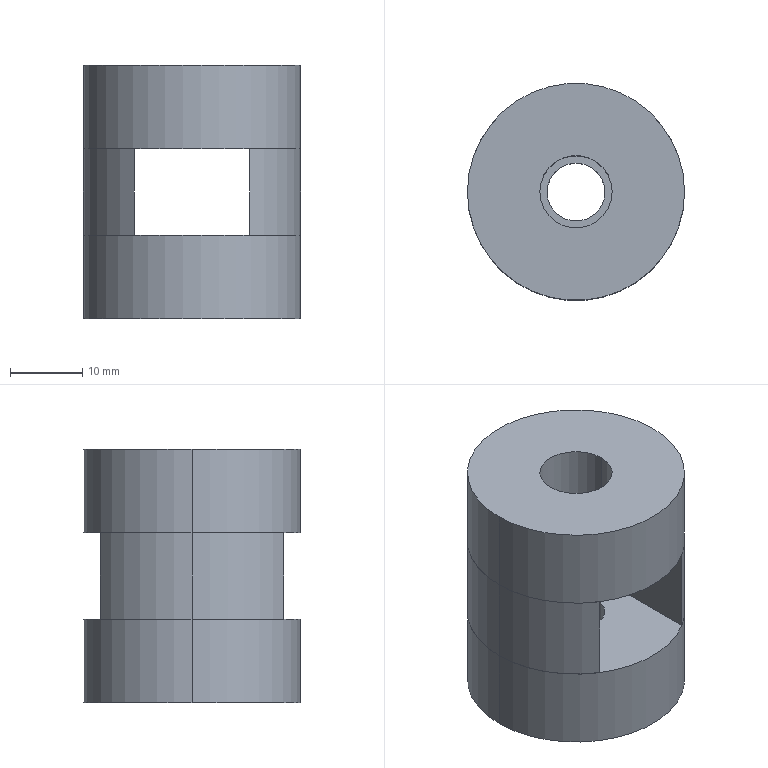Part | SolidWorks | features ICE 2, Extrusion 1, Split 1 | 4 solids | 21 faces | box 30 x 30 x 35 mm | volume 17785 mm3 | cylinder 11 | plane 10 | commonest cylinder face diameters 30 x7 8 x2 10 x2
STEP:
#1=CARTESIAN_POINT('',(8.,-12.689,6.));
#2=VERTEX_POINT('',#1);
#3=CARTESIAN_POINT('',(8.,12.689,6.));
#4=VERTEX_POINT('',#3);
#5=CARTESIAN_POINT('',(0.,0.,6.));
#6=DIRECTION('',(0.,0.,1.));
#7=DIRECTION('',(1.,0.,0.));
#8=AXIS2_PLACEMENT_3D('',#5,#6,#7);
#9=CIRCLE('',#8,15.);
#10=EDGE_CURVE('',#2,#4,#9,.T.);
#11=ORIENTED_EDGE('',*,*,#10,.T.);
#12=CARTESIAN_POINT('',(8.,-17.5,6.));
#13=DIRECTION('',(0.,1.,0.));
#14=VECTOR('',#13,1000.);
#15=LINE('',#12,#14);
#16=EDGE_CURVE('',#2,#4,#15,.T.);
#17=ORIENTED_EDGE('',*,*,#16,.F.);
#18=EDGE_LOOP('',(#11,#17));
#19=FACE_OUTER_BOUND('',#18,.T.);
#20=CARTESIAN_POINT('',(-15.,-15.01,6.));
#21=DIRECTION('',(0.,0.,1.));
#22=DIRECTION('',(1.,0.,0.));
#23=AXIS2_PLACEMENT_3D('',#20,#21,#22);
#24=PLANE('',#23);
#25=ADVANCED_FACE('',(#19),#24,.T.);
#26=CARTESIAN_POINT('',(8.,-12.689,-6.));
#27=VERTEX_POINT('',#26);
#28=CARTESIAN_POINT('',(8.,12.689,-6.));
#29=VERTEX_POINT('',#28);
#30=CARTESIAN_POINT('',(8.,-17.5,-6.));
#31=DIRECTION('',(0.,1.,0.));
#32=VECTOR('',#31,1000.);
#33=LINE('',#30,#32);
#34=EDGE_CURVE('',#27,#29,#33,.T.);
#35=ORIENTED_EDGE('',*,*,#34,.T.);
#36=CARTESIAN_POINT('',(0.,0.,-6.));
#37=DIRECTION('',(0.,0.,-1.));
#38=DIRECTION('',(-1.,0.,0.));
#39=AXIS2_PLACEMENT_3D('',#36,#37,#38);
#40=CIRCLE('',#39,15.);
#41=EDGE_CURVE('',#29,#27,#40,.T.);
#42=ORIENTED_EDGE('',*,*,#41,.T.);
#43=EDGE_LOOP('',(#35,#42));
#44=FACE_OUTER_BOUND('',#43,.T.);
#45=CARTESIAN_POINT('',(-15.,-15.01,-6.));
#46=DIRECTION('',(0.,0.,-1.));
#47=DIRECTION('',(-1.,0.,0.));
#48=AXIS2_PLACEMENT_3D('',#45,#46,#47);
#49=PLANE('',#48);
#50=ADVANCED_FACE('',(#44),#49,.T.);
#51=ORIENTED_EDGE('',*,*,#16,.T.);
#52=CARTESIAN_POINT('',(8.,12.689,17.5));
#53=DIRECTION('',(0.,0.,1.));
#54=VECTOR('',#53,1000.);
#55=LINE('',#52,#54);
#56=EDGE_CURVE('',#29,#4,#55,.T.);
#57=ORIENTED_EDGE('',*,*,#56,.F.);
#58=ORIENTED_EDGE('',*,*,#34,.F.);
#59=CARTESIAN_POINT('',(8.,-12.689,17.5));
#60=DIRECTION('',(0.,0.,-1.));
#61=VECTOR('',#60,1000.);
#62=LINE('',#59,#61);
#63=EDGE_CURVE('',#2,#27,#62,.T.);
#64=ORIENTED_EDGE('',*,*,#63,.F.);
#65=EDGE_LOOP('',(#51,#57,#58,#64));
#66=FACE_OUTER_BOUND('',#65,.T.);
#67=CARTESIAN_POINT('',(8.,-17.5,6.));
#68=DIRECTION('',(1.,0.,0.));
#69=DIRECTION('',(0.,0.,-1.));
#70=AXIS2_PLACEMENT_3D('',#67,#68,#69);
#71=PLANE('',#70);
#72=ADVANCED_FACE('',(#66),#71,.F.);
#73=ORIENTED_EDGE('',*,*,#56,.T.);
#74=ORIENTED_EDGE('',*,*,#10,.F.);
#75=ORIENTED_EDGE('',*,*,#63,.T.);
#76=ORIENTED_EDGE('',*,*,#41,.F.);
#77=EDGE_LOOP('',(#73,#74,#75,#76));
#78=FACE_OUTER_BOUND('',#77,.T.);
#79=CARTESIAN_POINT('',(0.,0.,17.5));
#80=DIRECTION('',(0.,0.,-1.));
#81=DIRECTION('',(-1.,0.,0.));
#82=AXIS2_PLACEMENT_3D('',#79,#80,#81);
#83=CYLINDRICAL_SURFACE('',#82,15.);
#84=ADVANCED_FACE('',(#78),#83,.T.);
#85=CLOSED_SHELL('',(#25,#50,#72,#84));
#86=MANIFOLD_SOLID_BREP('',#85);
#87=CARTESIAN_POINT('',(15.,0.,17.5));
#88=VERTEX_POINT('',#87);
#89=CARTESIAN_POINT('',(-15.,0.,17.5));
#90=VERTEX_POINT('',#89);
#91=CARTESIAN_POINT('',(0.,0.,17.5));
#92=DIRECTION('',(0.,0.,1.));
#93=DIRECTION('',(1.,0.,0.));
#94=AXIS2_PLACEMENT_3D('',#91,#92,#93);
#95=CIRCLE('',#94,15.);
#96=EDGE_CURVE('',#88,#90,#95,.T.);
#97=ORIENTED_EDGE('',*,*,#96,.F.);
#98=CARTESIAN_POINT('',(15.,0.,6.));
#99=VERTEX_POINT('',#98);
#100=CARTESIAN_POINT('',(15.,0.,17.5));
#101=DIRECTION('',(0.,0.,-1.));
#102=VECTOR('',#101,1000.);
#103=LINE('',#100,#102);
#104=EDGE_CURVE('',#88,#99,#103,.T.);
#105=ORIENTED_EDGE('',*,*,#104,.T.);
#106=CARTESIAN_POINT('',(-15.,0.,6.));
#107=VERTEX_POINT('',#106);
#108=CARTESIAN_POINT('',(0.,0.,6.));
#109=DIRECTION('',(0.,0.,1.));
#110=DIRECTION('',(1.,0.,0.));
#111=AXIS2_PLACEMENT_3D('',#108,#109,#110);
#112=CIRCLE('',#111,15.);
#113=EDGE_CURVE('',#99,#107,#112,.T.);
#114=ORIENTED_EDGE('',*,*,#113,.T.);
#115=CARTESIAN_POINT('',(-15.,0.,17.5));
#116=DIRECTION('',(0.,0.,-1.));
#117=VECTOR('',#116,1000.);
#118=LINE('',#115,#117);
#119=EDGE_CURVE('',#90,#107,#118,.T.);
#120=ORIENTED_EDGE('',*,*,#119,.F.);
#121=EDGE_LOOP('',(#97,#105,#114,#120));
#122=FACE_OUTER_BOUND('',#121,.T.);
#123=CARTESIAN_POINT('',(0.,0.,17.5));
#124=DIRECTION('',(0.,0.,-1.));
#125=DIRECTION('',(-1.,0.,0.));
#126=AXIS2_PLACEMENT_3D('',#123,#124,#125);
#127=CYLINDRICAL_SURFACE('',#126,15.);
#128=ADVANCED_FACE('',(#122),#127,.T.);
#129=CARTESIAN_POINT('',(5.,0.,6.));
#130=VERTEX_POINT('',#129);
#131=CARTESIAN_POINT('',(-5.,0.,6.));
#132=VERTEX_POINT('',#131);
#133=CARTESIAN_POINT('',(0.,0.,6.));
#134=DIRECTION('',(0.,0.,-1.));
#135=DIRECTION('',(1.,0.,0.));
#136=AXIS2_PLACEMENT_3D('',#133,#134,#135);
#137=CIRCLE('',#136,5.);
#138=EDGE_CURVE('',#130,#132,#137,.T.);
#139=ORIENTED_EDGE('',*,*,#138,.T.);
#140=CARTESIAN_POINT('',(-5.,0.,17.5));
#141=VERTEX_POINT('',#140);
#142=CARTESIAN_POINT('',(-5.,0.,-17.501));
#143=DIRECTION('',(0.,0.,1.));
#144=VECTOR('',#143,1000.);
#145=LINE('',#142,#144);
#146=EDGE_CURVE('',#132,#141,#145,.T.);
#147=ORIENTED_EDGE('',*,*,#146,.T.);
#148=CARTESIAN_POINT('',(5.,0.,17.5));
#149=VERTEX_POINT('',#148);
#150=CARTESIAN_POINT('',(0.,0.,17.5));
#151=DIRECTION('',(0.,0.,1.));
#152=DIRECTION('',(1.,0.,0.));
#153=AXIS2_PLACEMENT_3D('',#150,#151,#152);
#154=CIRCLE('',#153,5.);
#155=EDGE_CURVE('',#141,#149,#154,.T.);
#156=ORIENTED_EDGE('',*,*,#155,.T.);
#157=CARTESIAN_POINT('',(5.,0.,-17.501));
#158=DIRECTION('',(0.,0.,1.));
#159=VECTOR('',#158,1000.);
#160=LINE('',#157,#159);
#161=EDGE_CURVE('',#130,#149,#160,.T.);
#162=ORIENTED_EDGE('',*,*,#161,.F.);
#163=EDGE_LOOP('',(#139,#147,#156,#162));
#164=FACE_OUTER_BOUND('',#163,.T.);
#165=CARTESIAN_POINT('',(0.,0.,-17.501));
#166=DIRECTION('',(0.,0.,1.));
#167=DIRECTION('',(1.,0.,0.));
#168=AXIS2_PLACEMENT_3D('',#165,#166,#167);
#169=CYLINDRICAL_SURFACE('',#168,5.);
#170=ADVANCED_FACE('',(#164),#169,.F.);
#171=CARTESIAN_POINT('',(0.,0.,6.));
#172=DIRECTION('',(0.,0.,1.));
#173=DIRECTION('',(1.,0.,0.));
#174=AXIS2_PLACEMENT_3D('',#171,#172,#173);
#175=CIRCLE('',#174,15.);
#176=EDGE_CURVE('',#107,#99,#175,.T.);
#177=ORIENTED_EDGE('',*,*,#176,.F.);
#178=ORIENTED_EDGE('',*,*,#113,.F.);
#179=EDGE_LOOP('',(#177,#178));
#180=FACE_OUTER_BOUND('',#179,.T.);
#181=ORIENTED_EDGE('',*,*,#138,.F.);
#182=CARTESIAN_POINT('',(0.,0.,6.));
#183=DIRECTION('',(0.,0.,-1.));
#184=DIRECTION('',(1.,0.,0.));
#185=AXIS2_PLACEMENT_3D('',#182,#183,#184);
#186=CIRCLE('',#185,5.);
#187=EDGE_CURVE('',#132,#130,#186,.T.);
#188=ORIENTED_EDGE('',*,*,#187,.F.);
#189=EDGE_LOOP('',(#181,#188));
#190=FACE_BOUND('',#189,.T.);
#191=CARTESIAN_POINT('',(-15.,-15.01,6.));
#192=DIRECTION('',(0.,0.,1.));
#193=DIRECTION('',(1.,0.,0.));
#194=AXIS2_PLACEMENT_3D('',#191,#192,#193);
#195=PLANE('',#194);
#196=ADVANCED_FACE('',(#180,#190),#195,.F.);
#197=ORIENTED_EDGE('',*,*,#104,.F.);
#198=CARTESIAN_POINT('',(0.,0.,17.5));
#199=DIRECTION('',(0.,0.,1.));
#200=DIRECTION('',(1.,0.,0.));
#201=AXIS2_PLACEMENT_3D('',#198,#199,#200);
#202=CIRCLE('',#201,15.);
#203=EDGE_CURVE('',#90,#88,#202,.T.);
#204=ORIENTED_EDGE('',*,*,#203,.F.);
#205=ORIENTED_EDGE('',*,*,#119,.T.);
#206=ORIENTED_EDGE('',*,*,#176,.T.);
#207=EDGE_LOOP('',(#197,#204,#205,#206));
#208=FACE_OUTER_BOUND('',#207,.T.);
#209=CARTESIAN_POINT('',(0.,0.,17.5));
#210=DIRECTION('',(0.,0.,-1.));
#211=DIRECTION('',(-1.,0.,0.));
#212=AXIS2_PLACEMENT_3D('',#209,#210,#211);
#213=CYLINDRICAL_SURFACE('',#212,15.);
#214=ADVANCED_FACE('',(#208),#213,.T.);
#215=ORIENTED_EDGE('',*,*,#146,.F.);
#216=ORIENTED_EDGE('',*,*,#187,.T.);
#217=ORIENTED_EDGE('',*,*,#161,.T.);
#218=CARTESIAN_POINT('',(0.,0.,17.5));
#219=DIRECTION('',(0.,0.,1.));
#220=DIRECTION('',(1.,0.,0.));
#221=AXIS2_PLACEMENT_3D('',#218,#219,#220);
#222=CIRCLE('',#221,5.);
#223=EDGE_CURVE('',#149,#141,#222,.T.);
#224=ORIENTED_EDGE('',*,*,#223,.T.);
#225=EDGE_LOOP('',(#215,#216,#217,#224));
#226=FACE_OUTER_BOUND('',#225,.T.);
#227=CARTESIAN_POINT('',(0.,0.,-17.501));
#228=DIRECTION('',(0.,0.,1.));
#229=DIRECTION('',(1.,0.,0.));
#230=AXIS2_PLACEMENT_3D('',#227,#228,#229);
#231=CYLINDRICAL_SURFACE('',#230,5.);
#232=ADVANCED_FACE('',(#226),#231,.F.);
#233=ORIENTED_EDGE('',*,*,#223,.F.);
#234=ORIENTED_EDGE('',*,*,#155,.F.);
#235=EDGE_LOOP('',(#233,#234));
#236=FACE_BOUND('',#235,.T.);
#237=ORIENTED_EDGE('',*,*,#203,.T.);
#238=ORIENTED_EDGE('',*,*,#96,.T.);
#239=EDGE_LOOP('',(#237,#238));
#240=FACE_OUTER_BOUND('',#239,.T.);
#241=CARTESIAN_POINT('',(0.,0.,17.5));
#242=DIRECTION('',(0.,0.,1.));
#243=DIRECTION('',(1.,0.,0.));
#244=AXIS2_PLACEMENT_3D('',#241,#242,#243);
#245=PLANE('',#244);
#246=ADVANCED_FACE('',(#236,#240),#245,.T.);
#247=CLOSED_SHELL('',(#128,#170,#196,#214,#232,#246));
#248=MANIFOLD_SOLID_BREP('',#247);
#249=CARTESIAN_POINT('',(4.,0.,-6.));
#250=VERTEX_POINT('',#249);
#251=CARTESIAN_POINT('',(-4.,0.,-6.));
#252=VERTEX_POINT('',#251);
#253=CARTESIAN_POINT('',(0.,0.,-6.));
#254=DIRECTION('',(0.,0.,-1.));
#255=DIRECTION('',(-1.,0.,0.));
#256=AXIS2_PLACEMENT_3D('',#253,#254,#255);
#257=CIRCLE('',#256,4.);
#258=EDGE_CURVE('',#250,#252,#257,.T.);
#259=ORIENTED_EDGE('',*,*,#258,.F.);
#260=CARTESIAN_POINT('',(4.,0.,-17.5));
#261=VERTEX_POINT('',#260);
#262=CARTESIAN_POINT('',(4.,0.,17.5));
#263=DIRECTION('',(0.,0.,-1.));
#264=VECTOR('',#263,1000.);
#265=LINE('',#262,#264);
#266=EDGE_CURVE('',#250,#261,#265,.T.);
#267=ORIENTED_EDGE('',*,*,#266,.T.);
#268=CARTESIAN_POINT('',(-4.,0.,-17.5));
#269=VERTEX_POINT('',#268);
#270=CARTESIAN_POINT('',(0.,0.,-17.5));
#271=DIRECTION('',(0.,0.,1.));
#272=DIRECTION('',(1.,0.,0.));
#273=AXIS2_PLACEMENT_3D('',#270,#271,#272);
#274=CIRCLE('',#273,4.);
#275=EDGE_CURVE('',#269,#261,#274,.T.);
#276=ORIENTED_EDGE('',*,*,#275,.F.);
#277=CARTESIAN_POINT('',(-4.,0.,17.5));
#278=DIRECTION('',(0.,0.,-1.));
#279=VECTOR('',#278,1000.);
#280=LINE('',#277,#279);
#281=EDGE_CURVE('',#252,#269,#280,.T.);
#282=ORIENTED_EDGE('',*,*,#281,.F.);
#283=EDGE_LOOP('',(#259,#267,#276,#282));
#284=FACE_OUTER_BOUND('',#283,.T.);
#285=CARTESIAN_POINT('',(0.,0.,17.5));
#286=DIRECTION('',(0.,0.,-1.));
#287=DIRECTION('',(-1.,0.,0.));
#288=AXIS2_PLACEMENT_3D('',#285,#286,#287);
#289=CYLINDRICAL_SURFACE('',#288,4.);
#290=ADVANCED_FACE('',(#284),#289,.F.);
#291=CARTESIAN_POINT('',(-15.,0.,-6.));
#292=VERTEX_POINT('',#291);
#293=CARTESIAN_POINT('',(15.,0.,-6.));
#294=VERTEX_POINT('',#293);
#295=CARTESIAN_POINT('',(0.,0.,-6.));
#296=DIRECTION('',(0.,0.,-1.));
#297=DIRECTION('',(-1.,0.,0.));
#298=AXIS2_PLACEMENT_3D('',#295,#296,#297);
#299=CIRCLE('',#298,15.);
#300=EDGE_CURVE('',#292,#294,#299,.T.);
#301=ORIENTED_EDGE('',*,*,#300,.T.);
#302=CARTESIAN_POINT('',(15.,0.,-17.5));
#303=VERTEX_POINT('',#302);
#304=CARTESIAN_POINT('',(15.,0.,17.5));
#305=DIRECTION('',(0.,0.,-1.));
#306=VECTOR('',#305,1000.);
#307=LINE('',#304,#306);
#308=EDGE_CURVE('',#294,#303,#307,.T.);
#309=ORIENTED_EDGE('',*,*,#308,.T.);
#310=CARTESIAN_POINT('',(-15.,0.,-17.5));
#311=VERTEX_POINT('',#310);
#312=CARTESIAN_POINT('',(0.,0.,-17.5));
#313=DIRECTION('',(0.,0.,1.));
#314=DIRECTION('',(1.,0.,0.));
#315=AXIS2_PLACEMENT_3D('',#312,#313,#314);
#316=CIRCLE('',#315,15.);
#317=EDGE_CURVE('',#303,#311,#316,.T.);
#318=ORIENTED_EDGE('',*,*,#317,.T.);
#319=CARTESIAN_POINT('',(-15.,0.,17.5));
#320=DIRECTION('',(0.,0.,-1.));
#321=VECTOR('',#320,1000.);
#322=LINE('',#319,#321);
#323=EDGE_CURVE('',#292,#311,#322,.T.);
#324=ORIENTED_EDGE('',*,*,#323,.F.);
#325=EDGE_LOOP('',(#301,#309,#318,#324));
#326=FACE_OUTER_BOUND('',#325,.T.);
#327=CARTESIAN_POINT('',(0.,0.,17.5));
#328=DIRECTION('',(0.,0.,-1.));
#329=DIRECTION('',(-1.,0.,0.));
#330=AXIS2_PLACEMENT_3D('',#327,#328,#329);
#331=CYLINDRICAL_SURFACE('',#330,15.);
#332=ADVANCED_FACE('',(#326),#331,.T.);
#333=ORIENTED_EDGE('',*,*,#300,.F.);
#334=CARTESIAN_POINT('',(0.,0.,-6.));
#335=DIRECTION('',(0.,0.,-1.));
#336=DIRECTION('',(-1.,0.,0.));
#337=AXIS2_PLACEMENT_3D('',#334,#335,#336);
#338=CIRCLE('',#337,15.);
#339=EDGE_CURVE('',#294,#292,#338,.T.);
#340=ORIENTED_EDGE('',*,*,#339,.F.);
#341=EDGE_LOOP('',(#333,#340));
#342=FACE_OUTER_BOUND('',#341,.T.);
#343=CARTESIAN_POINT('',(0.,0.,-6.));
#344=DIRECTION('',(0.,0.,-1.));
#345=DIRECTION('',(-1.,0.,0.));
#346=AXIS2_PLACEMENT_3D('',#343,#344,#345);
#347=CIRCLE('',#346,4.);
#348=EDGE_CURVE('',#252,#250,#347,.T.);
#349=ORIENTED_EDGE('',*,*,#348,.T.);
#350=ORIENTED_EDGE('',*,*,#258,.T.);
#351=EDGE_LOOP('',(#349,#350));
#352=FACE_BOUND('',#351,.T.);
#353=CARTESIAN_POINT('',(-15.,-15.01,-6.));
#354=DIRECTION('',(0.,0.,-1.));
#355=DIRECTION('',(-1.,0.,0.));
#356=AXIS2_PLACEMENT_3D('',#353,#354,#355);
#357=PLANE('',#356);
#358=ADVANCED_FACE('',(#342,#352),#357,.F.);
#359=ORIENTED_EDGE('',*,*,#266,.F.);
#360=ORIENTED_EDGE('',*,*,#348,.F.);
#361=ORIENTED_EDGE('',*,*,#281,.T.);
#362=CARTESIAN_POINT('',(0.,0.,-17.5));
#363=DIRECTION('',(0.,0.,1.));
#364=DIRECTION('',(1.,0.,0.));
#365=AXIS2_PLACEMENT_3D('',#362,#363,#364);
#366=CIRCLE('',#365,4.);
#367=EDGE_CURVE('',#261,#269,#366,.T.);
#368=ORIENTED_EDGE('',*,*,#367,.F.);
#369=EDGE_LOOP('',(#359,#360,#361,#368));
#370=FACE_OUTER_BOUND('',#369,.T.);
#371=CARTESIAN_POINT('',(0.,0.,17.5));
#372=DIRECTION('',(0.,0.,-1.));
#373=DIRECTION('',(-1.,0.,0.));
#374=AXIS2_PLACEMENT_3D('',#371,#372,#373);
#375=CYLINDRICAL_SURFACE('',#374,4.);
#376=ADVANCED_FACE('',(#370),#375,.F.);
#377=ORIENTED_EDGE('',*,*,#308,.F.);
#378=ORIENTED_EDGE('',*,*,#339,.T.);
#379=ORIENTED_EDGE('',*,*,#323,.T.);
#380=CARTESIAN_POINT('',(0.,0.,-17.5));
#381=DIRECTION('',(0.,0.,1.));
#382=DIRECTION('',(1.,0.,0.));
#383=AXIS2_PLACEMENT_3D('',#380,#381,#382);
#384=CIRCLE('',#383,15.);
#385=EDGE_CURVE('',#311,#303,#384,.T.);
#386=ORIENTED_EDGE('',*,*,#385,.T.);
#387=EDGE_LOOP('',(#377,#378,#379,#386));
#388=FACE_OUTER_BOUND('',#387,.T.);
#389=CARTESIAN_POINT('',(0.,0.,17.5));
#390=DIRECTION('',(0.,0.,-1.));
#391=DIRECTION('',(-1.,0.,0.));
#392=AXIS2_PLACEMENT_3D('',#389,#390,#391);
#393=CYLINDRICAL_SURFACE('',#392,15.);
#394=ADVANCED_FACE('',(#388),#393,.T.);
#395=ORIENTED_EDGE('',*,*,#385,.F.);
#396=ORIENTED_EDGE('',*,*,#317,.F.);
#397=EDGE_LOOP('',(#395,#396));
#398=FACE_OUTER_BOUND('',#397,.T.);
#399=ORIENTED_EDGE('',*,*,#275,.T.);
#400=ORIENTED_EDGE('',*,*,#367,.T.);
#401=EDGE_LOOP('',(#399,#400));
#402=FACE_BOUND('',#401,.T.);
#403=CARTESIAN_POINT('',(0.,0.,-17.5));
#404=DIRECTION('',(0.,0.,1.));
#405=DIRECTION('',(1.,0.,0.));
#406=AXIS2_PLACEMENT_3D('',#403,#404,#405);
#407=PLANE('',#406);
#408=ADVANCED_FACE('',(#398,#402),#407,.F.);
#409=CLOSED_SHELL('',(#290,#332,#358,#376,#394,#408));
#410=MANIFOLD_SOLID_BREP('',#409);
#411=CARTESIAN_POINT('',(-15.,0.,6.));
#412=VERTEX_POINT('',#411);
#413=CARTESIAN_POINT('',(-8.,-12.689,6.));
#414=VERTEX_POINT('',#413);
#415=CARTESIAN_POINT('',(0.,0.,6.));
#416=DIRECTION('',(0.,0.,1.));
#417=DIRECTION('',(1.,0.,0.));
#418=AXIS2_PLACEMENT_3D('',#415,#416,#417);
#419=CIRCLE('',#418,15.);
#420=EDGE_CURVE('',#412,#414,#419,.T.);
#421=ORIENTED_EDGE('',*,*,#420,.F.);
#422=CARTESIAN_POINT('',(-15.,0.,-6.));
#423=VERTEX_POINT('',#422);
#424=CARTESIAN_POINT('',(-15.,0.,17.5));
#425=DIRECTION('',(0.,0.,-1.));
#426=VECTOR('',#425,1000.);
#427=LINE('',#424,#426);
#428=EDGE_CURVE('',#412,#423,#427,.T.);
#429=ORIENTED_EDGE('',*,*,#428,.T.);
#430=CARTESIAN_POINT('',(-8.,-12.689,-6.));
#431=VERTEX_POINT('',#430);
#432=CARTESIAN_POINT('',(0.,0.,-6.));
#433=DIRECTION('',(0.,0.,-1.));
#434=DIRECTION('',(-1.,0.,0.));
#435=AXIS2_PLACEMENT_3D('',#432,#433,#434);
#436=CIRCLE('',#435,15.);
#437=EDGE_CURVE('',#431,#423,#436,.T.);
#438=ORIENTED_EDGE('',*,*,#437,.F.);
#439=CARTESIAN_POINT('',(-8.,-12.689,17.5));
#440=DIRECTION('',(0.,0.,1.));
#441=VECTOR('',#440,1000.);
#442=LINE('',#439,#441);
#443=EDGE_CURVE('',#431,#414,#442,.T.);
#444=ORIENTED_EDGE('',*,*,#443,.T.);
#445=EDGE_LOOP('',(#421,#429,#438,#444));
#446=FACE_OUTER_BOUND('',#445,.T.);
#447=CARTESIAN_POINT('',(0.,0.,17.5));
#448=DIRECTION('',(0.,0.,-1.));
#449=DIRECTION('',(-1.,0.,0.));
#450=AXIS2_PLACEMENT_3D('',#447,#448,#449);
#451=CYLINDRICAL_SURFACE('',#450,15.);
#452=ADVANCED_FACE('',(#446),#451,.T.);
#453=ORIENTED_EDGE('',*,*,#428,.F.);
#454=CARTESIAN_POINT('',(-8.,12.689,6.));
#455=VERTEX_POINT('',#454);
#456=CARTESIAN_POINT('',(0.,0.,6.));
#457=DIRECTION('',(0.,0.,1.));
#458=DIRECTION('',(1.,0.,0.));
#459=AXIS2_PLACEMENT_3D('',#456,#457,#458);
#460=CIRCLE('',#459,15.);
#461=EDGE_CURVE('',#455,#412,#460,.T.);
#462=ORIENTED_EDGE('',*,*,#461,.F.);
#463=CARTESIAN_POINT('',(-8.,12.689,-6.));
#464=VERTEX_POINT('',#463);
#465=CARTESIAN_POINT('',(-8.,12.689,17.5));
#466=DIRECTION('',(0.,0.,-1.));
#467=VECTOR('',#466,1000.);
#468=LINE('',#465,#467);
#469=EDGE_CURVE('',#455,#464,#468,.T.);
#470=ORIENTED_EDGE('',*,*,#469,.T.);
#471=CARTESIAN_POINT('',(0.,0.,-6.));
#472=DIRECTION('',(0.,0.,-1.));
#473=DIRECTION('',(-1.,0.,0.));
#474=AXIS2_PLACEMENT_3D('',#471,#472,#473);
#475=CIRCLE('',#474,15.);
#476=EDGE_CURVE('',#423,#464,#475,.T.);
#477=ORIENTED_EDGE('',*,*,#476,.F.);
#478=EDGE_LOOP('',(#453,#462,#470,#477));
#479=FACE_OUTER_BOUND('',#478,.T.);
#480=CARTESIAN_POINT('',(0.,0.,17.5));
#481=DIRECTION('',(0.,0.,-1.));
#482=DIRECTION('',(-1.,0.,0.));
#483=AXIS2_PLACEMENT_3D('',#480,#481,#482);
#484=CYLINDRICAL_SURFACE('',#483,15.);
#485=ADVANCED_FACE('',(#479),#484,.T.);
#486=CARTESIAN_POINT('',(-8.,-17.5,6.));
#487=DIRECTION('',(0.,1.,0.));
#488=VECTOR('',#487,1000.);
#489=LINE('',#486,#488);
#490=EDGE_CURVE('',#414,#455,#489,.T.);
#491=ORIENTED_EDGE('',*,*,#490,.F.);
#492=ORIENTED_EDGE('',*,*,#443,.F.);
#493=CARTESIAN_POINT('',(-8.,-17.5,-6.));
#494=DIRECTION('',(0.,1.,0.));
#495=VECTOR('',#494,1000.);
#496=LINE('',#493,#495);
#497=EDGE_CURVE('',#431,#464,#496,.T.);
#498=ORIENTED_EDGE('',*,*,#497,.T.);
#499=ORIENTED_EDGE('',*,*,#469,.F.);
#500=EDGE_LOOP('',(#491,#492,#498,#499));
#501=FACE_OUTER_BOUND('',#500,.T.);
#502=CARTESIAN_POINT('',(-8.,-17.5,6.));
#503=DIRECTION('',(-1.,0.,0.));
#504=DIRECTION('',(0.,0.,1.));
#505=AXIS2_PLACEMENT_3D('',#502,#503,#504);
#506=PLANE('',#505);
#507=ADVANCED_FACE('',(#501),#506,.F.);
#508=ORIENTED_EDGE('',*,*,#437,.T.);
#509=ORIENTED_EDGE('',*,*,#476,.T.);
#510=ORIENTED_EDGE('',*,*,#497,.F.);
#511=EDGE_LOOP('',(#508,#509,#510));
#512=FACE_OUTER_BOUND('',#511,.T.);
#513=CARTESIAN_POINT('',(-15.,-15.01,-6.));
#514=DIRECTION('',(0.,0.,-1.));
#515=DIRECTION('',(-1.,0.,0.));
#516=AXIS2_PLACEMENT_3D('',#513,#514,#515);
#517=PLANE('',#516);
#518=ADVANCED_FACE('',(#512),#517,.T.);
#519=ORIENTED_EDGE('',*,*,#490,.T.);
#520=ORIENTED_EDGE('',*,*,#461,.T.);
#521=ORIENTED_EDGE('',*,*,#420,.T.);
#522=EDGE_LOOP('',(#519,#520,#521));
#523=FACE_OUTER_BOUND('',#522,.T.);
#524=CARTESIAN_POINT('',(-15.,-15.01,6.));
#525=DIRECTION('',(0.,0.,1.));
#526=DIRECTION('',(1.,0.,0.));
#527=AXIS2_PLACEMENT_3D('',#524,#525,#526);
#528=PLANE('',#527);
#529=ADVANCED_FACE('',(#523),#528,.T.);
#530=CLOSED_SHELL('',(#452,#485,#507,#518,#529));
#531=MANIFOLD_SOLID_BREP('',#530);
#532=CARTESIAN_POINT('',(0.,0.,0.));
#533=DIRECTION('',(0.,0.,1.));
#534=DIRECTION('',(1.,0.,0.));
#535=AXIS2_PLACEMENT_3D('',#532,#533,#534);
#536=(LENGTH_UNIT()NAMED_UNIT(*)SI_UNIT(.MILLI.,.METRE.));
#537=UNCERTAINTY_MEASURE_WITH_UNIT(LENGTH_MEASURE(0.00001),#536,'','');
#538=(NAMED_UNIT(*)PLANE_ANGLE_UNIT()SI_UNIT($,.RADIAN.));
#539=(NAMED_UNIT(*)SI_UNIT($,.STERADIAN.)SOLID_ANGLE_UNIT());
#540=(GEOMETRIC_REPRESENTATION_CONTEXT(3)GLOBAL_UNCERTAINTY_ASSIGNED_CONTEXT((#537))GLOBAL_UNIT_ASSIGNED_CONTEXT((#536,#538,#539))REPRESENTATION_CONTEXT('',''));
#541=ADVANCED_BREP_SHAPE_REPRESENTATION('',(#86,#248,#410,#531,#535),#540);